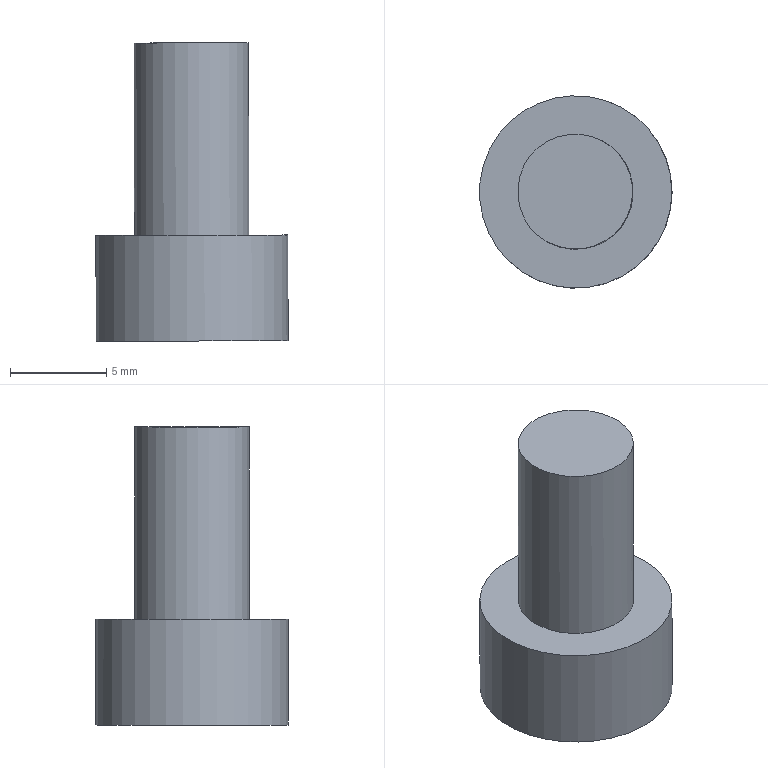Part | NX | features solid 2 | 1 solid | 12 faces | box 10.013 x 10.001 x 15.519 mm | volume 621.654 mm3 | plane 10 | spline 1 | cylinder 1 | commonest cylinder face diameters 10 x1
STEP:
#1=CARTESIAN_POINT('',(-491.131,18.224,140.018));
#2=VERTEX_POINT('',#1);
#3=CARTESIAN_POINT('',(-492.412,20.286,140.015));
#4=CARTESIAN_POINT('',(-491.355,17.975,140.017));
#5=CARTESIAN_POINT('',(-488.952,17.156,140.023));
#6=CARTESIAN_POINT('',(-486.649,18.209,140.028));
#7=CARTESIAN_POINT('',(-485.825,20.612,140.031));
#8=CARTESIAN_POINT('',(-486.88,22.919,140.029));
#9=CARTESIAN_POINT('',(-489.28,23.741,140.023));
#10=CARTESIAN_POINT('',(-491.587,22.69,140.018));
#11=CARTESIAN_POINT('',(-492.412,20.286,140.015));
#12=CARTESIAN_POINT('',(-491.355,17.975,140.017));
#13=CARTESIAN_POINT('',(-488.952,17.156,140.023));
#14=B_SPLINE_CURVE_WITH_KNOTS('',3,(#3,#4,#5,#6,#7,#8,#9,#10,#11,#12,#13),.UNSPECIFIED.,.T.,.F.,(1,1,1,1,1,1,1,1,1,1,1,1,1,1,1),(-0.007013,-0.004676,-0.002338,0.,0.002338,0.004676,0.007013,0.009351,0.01169,0.01403,0.01636,0.0187,0.02104,0.02338,0.02572),.UNSPECIFIED.);
#15=EDGE_CURVE('',#2,#2,#14,.T.);
#16=ORIENTED_EDGE('',*,*,#15,.F.);
#17=EDGE_LOOP('',(#16));
#18=FACE_BOUND('',#17,.T.);
#19=CARTESIAN_POINT('',(-491.107,18.226,130.018));
#20=VERTEX_POINT('',#19);
#21=CARTESIAN_POINT('',(-492.388,20.288,130.015));
#22=CARTESIAN_POINT('',(-491.332,17.977,130.017));
#23=CARTESIAN_POINT('',(-488.928,17.158,130.023));
#24=CARTESIAN_POINT('',(-486.625,18.211,130.029));
#25=CARTESIAN_POINT('',(-485.801,20.614,130.031));
#26=CARTESIAN_POINT('',(-486.856,22.921,130.029));
#27=CARTESIAN_POINT('',(-489.256,23.743,130.023));
#28=CARTESIAN_POINT('',(-491.563,22.692,130.018));
#29=CARTESIAN_POINT('',(-492.388,20.288,130.015));
#30=CARTESIAN_POINT('',(-491.332,17.977,130.017));
#31=CARTESIAN_POINT('',(-488.928,17.158,130.023));
#32=B_SPLINE_CURVE_WITH_KNOTS('',3,(#21,#22,#23,#24,#25,#26,#27,#28,#29,#30,#31),.UNSPECIFIED.,.T.,.F.,(1,1,1,1,1,1,1,1,1,1,1,1,1,1,1),(-0.007013,-0.004676,-0.002338,0.,0.002338,0.004676,0.007013,0.009351,0.01169,0.01403,0.01636,0.0187,0.02104,0.02338,0.02572),.UNSPECIFIED.);
#33=EDGE_CURVE('',#20,#20,#32,.T.);
#34=ORIENTED_EDGE('',*,*,#33,.T.);
#35=EDGE_LOOP('',(#34));
#36=FACE_BOUND('',#35,.T.);
#37=CARTESIAN_POINT('',(-485.825,20.613,140.031));
#38=CARTESIAN_POINT('',(-485.802,20.615,130.031));
#39=CARTESIAN_POINT('',(-486.881,22.921,140.029));
#40=CARTESIAN_POINT('',(-486.857,22.923,130.029));
#41=CARTESIAN_POINT('',(-489.283,23.741,140.023));
#42=CARTESIAN_POINT('',(-489.259,23.743,130.023));
#43=CARTESIAN_POINT('',(-491.591,22.685,140.018));
#44=CARTESIAN_POINT('',(-491.567,22.687,130.018));
#45=CARTESIAN_POINT('',(-492.411,20.284,140.015));
#46=CARTESIAN_POINT('',(-492.387,20.286,130.015));
#47=CARTESIAN_POINT('',(-491.355,17.976,140.017));
#48=CARTESIAN_POINT('',(-491.331,17.978,130.017));
#49=CARTESIAN_POINT('',(-488.954,17.155,140.023));
#50=CARTESIAN_POINT('',(-488.93,17.157,130.023));
#51=CARTESIAN_POINT('',(-486.646,18.211,140.029));
#52=CARTESIAN_POINT('',(-486.622,18.213,130.029));
#53=CARTESIAN_POINT('',(-485.825,20.613,140.031));
#54=CARTESIAN_POINT('',(-485.802,20.615,130.031));
#55=CARTESIAN_POINT('',(-486.881,22.921,140.029));
#56=CARTESIAN_POINT('',(-486.857,22.923,130.029));
#57=CARTESIAN_POINT('',(-489.283,23.741,140.023));
#58=CARTESIAN_POINT('',(-489.259,23.743,130.023));
#59=B_SPLINE_SURFACE_WITH_KNOTS('',3,1,((#37,#38),(#39,#40),(#41,#42),(#43,#44),(#45,#46),(#47,#48),(#49,#50),(#51,#52),(#53,#54),(#55,#56),(#57,#58)),.SURF_OF_LINEAR_EXTRUSION.,.T.,.F.,.F.,(1,1,1,1,1,1,1,1,1,1,1,1,1,1,1),(2,2),(-0.375,-0.25,-0.125,0.,0.125,0.25,0.375,0.5,0.625,0.75,0.875,1.,1.125,1.25,1.375),(0.,1.),.UNSPECIFIED.);
#60=ADVANCED_FACE('',(#18,#36),#59,.F.);
#61=ORIENTED_EDGE('',*,*,#15,.T.);
#62=EDGE_LOOP('',(#61));
#63=FACE_BOUND('',#62,.T.);
#64=CARTESIAN_POINT('',(-491.802,17.482,140.016));
#65=DIRECTION('',(-0.002392,-0.0002093,1.));
#66=DIRECTION('',(-0.7415,0.6709,-0.001634));
#67=AXIS2_PLACEMENT_3D('',#64,#65,#66);
#68=PLANE('',#67);
#69=ADVANCED_FACE('',(#63),#68,.T.);
#70=CARTESIAN_POINT('',(-494.075,20.015,130.011));
#71=VERTEX_POINT('',#70);
#72=CARTESIAN_POINT('',(-489.094,20.45,130.023));
#73=DIRECTION('',(-0.002392,-0.0002093,1.));
#74=DIRECTION('',(-0.9962,-0.08716,-0.002401));
#75=AXIS2_PLACEMENT_3D('',#72,#73,#74);
#76=CIRCLE('',#75,5.);
#77=EDGE_CURVE('',#71,#71,#76,.T.);
#78=ORIENTED_EDGE('',*,*,#77,.F.);
#79=EDGE_LOOP('',(#78));
#80=FACE_BOUND('',#79,.T.);
#81=CARTESIAN_POINT('',(-494.062,20.016,124.511));
#82=VERTEX_POINT('',#81);
#83=CARTESIAN_POINT('',(-489.081,20.452,124.523));
#84=DIRECTION('',(-0.002392,-0.0002093,1.));
#85=DIRECTION('',(-0.9962,-0.08716,-0.002401));
#86=AXIS2_PLACEMENT_3D('',#83,#84,#85);
#87=CIRCLE('',#86,5.);
#88=EDGE_CURVE('',#82,#82,#87,.T.);
#89=ORIENTED_EDGE('',*,*,#88,.T.);
#90=EDGE_LOOP('',(#89));
#91=FACE_BOUND('',#90,.T.);
#92=CARTESIAN_POINT('',(-489.094,20.45,130.023));
#93=DIRECTION('',(0.002392,0.0002093,-1.));
#94=DIRECTION('',(0.7415,-0.6709,0.001634));
#95=AXIS2_PLACEMENT_3D('',#92,#93,#94);
#96=CYLINDRICAL_SURFACE('',#95,5.);
#97=ADVANCED_FACE('',(#80,#91),#96,.T.);
#98=ORIENTED_EDGE('',*,*,#33,.F.);
#99=EDGE_LOOP('',(#98));
#100=FACE_BOUND('',#99,.T.);
#101=ORIENTED_EDGE('',*,*,#77,.T.);
#102=EDGE_LOOP('',(#101));
#103=FACE_BOUND('',#102,.T.);
#104=CARTESIAN_POINT('',(-489.094,20.45,130.023));
#105=DIRECTION('',(0.002392,0.0002093,-1.));
#106=DIRECTION('',(0.7415,-0.6709,0.001634));
#107=AXIS2_PLACEMENT_3D('',#104,#105,#106);
#108=PLANE('',#107);
#109=ADVANCED_FACE('',(#100,#103),#108,.F.);
#110=CARTESIAN_POINT('',(-491.205,18.104,124.518));
#111=VERTEX_POINT('',#110);
#112=CARTESIAN_POINT('',(-488.11,17.439,124.525));
#113=VERTEX_POINT('',#112);
#114=CARTESIAN_POINT('',(-489.658,17.772,124.521));
#115=DIRECTION('',(0.9776,-0.2103,0.002295));
#116=VECTOR('',#115,1000.);
#117=LINE('',#114,#116);
#118=EDGE_CURVE('',#111,#113,#117,.T.);
#119=ORIENTED_EDGE('',*,*,#118,.T.);
#120=CARTESIAN_POINT('',(-485.987,19.786,124.53));
#121=VERTEX_POINT('',#120);
#122=CARTESIAN_POINT('',(-487.049,18.612,124.528));
#123=DIRECTION('',(0.6709,0.7415,0.00176));
#124=VECTOR('',#123,1000.);
#125=LINE('',#122,#124);
#126=EDGE_CURVE('',#113,#121,#125,.T.);
#127=ORIENTED_EDGE('',*,*,#126,.T.);
#128=CARTESIAN_POINT('',(-486.958,22.799,124.529));
#129=VERTEX_POINT('',#128);
#130=CARTESIAN_POINT('',(-486.472,21.292,124.53));
#131=DIRECTION('',(-0.3067,0.9518,-0.0005346));
#132=VECTOR('',#131,1000.);
#133=LINE('',#130,#132);
#134=EDGE_CURVE('',#121,#129,#133,.T.);
#135=ORIENTED_EDGE('',*,*,#134,.T.);
#136=CARTESIAN_POINT('',(-490.052,23.464,124.521));
#137=VERTEX_POINT('',#136);
#138=CARTESIAN_POINT('',(-488.505,23.132,124.525));
#139=DIRECTION('',(-0.9776,0.2103,-0.002295));
#140=VECTOR('',#139,1000.);
#141=LINE('',#138,#140);
#142=EDGE_CURVE('',#129,#137,#141,.T.);
#143=ORIENTED_EDGE('',*,*,#142,.T.);
#144=CARTESIAN_POINT('',(-492.176,21.117,124.516));
#145=VERTEX_POINT('',#144);
#146=CARTESIAN_POINT('',(-491.114,22.291,124.519));
#147=DIRECTION('',(-0.6709,-0.7415,-0.00176));
#148=VECTOR('',#147,1000.);
#149=LINE('',#146,#148);
#150=EDGE_CURVE('',#137,#145,#149,.T.);
#151=ORIENTED_EDGE('',*,*,#150,.T.);
#152=CARTESIAN_POINT('',(-491.69,19.611,124.517));
#153=DIRECTION('',(0.3067,-0.9518,0.0005346));
#154=VECTOR('',#153,1000.);
#155=LINE('',#152,#154);
#156=EDGE_CURVE('',#145,#111,#155,.T.);
#157=ORIENTED_EDGE('',*,*,#156,.T.);
#158=EDGE_LOOP('',(#119,#127,#135,#143,#151,#157));
#159=FACE_BOUND('',#158,.T.);
#160=ORIENTED_EDGE('',*,*,#88,.F.);
#161=EDGE_LOOP('',(#160));
#162=FACE_BOUND('',#161,.T.);
#163=CARTESIAN_POINT('',(-489.081,20.452,124.523));
#164=DIRECTION('',(0.002392,0.0002093,-1.));
#165=DIRECTION('',(0.7415,-0.6709,0.001634));
#166=AXIS2_PLACEMENT_3D('',#163,#164,#165);
#167=PLANE('',#166);
#168=ADVANCED_FACE('',(#159,#162),#167,.T.);
#169=ORIENTED_EDGE('',*,*,#118,.F.);
#170=CARTESIAN_POINT('',(-491.213,18.104,128.018));
#171=VERTEX_POINT('',#170);
#172=CARTESIAN_POINT('',(-491.213,18.104,128.018));
#173=DIRECTION('',(0.002392,0.0002093,-1.));
#174=VECTOR('',#173,1000.);
#175=LINE('',#172,#174);
#176=EDGE_CURVE('',#171,#111,#175,.T.);
#177=ORIENTED_EDGE('',*,*,#176,.F.);
#178=CARTESIAN_POINT('',(-488.119,17.438,128.025));
#179=VERTEX_POINT('',#178);
#180=CARTESIAN_POINT('',(-491.778,18.225,128.016));
#181=DIRECTION('',(0.9776,-0.2103,0.002295));
#182=VECTOR('',#181,1000.);
#183=LINE('',#180,#182);
#184=EDGE_CURVE('',#171,#179,#183,.T.);
#185=ORIENTED_EDGE('',*,*,#184,.T.);
#186=CARTESIAN_POINT('',(-488.119,17.438,128.025));
#187=DIRECTION('',(0.002392,0.0002093,-1.));
#188=VECTOR('',#187,1000.);
#189=LINE('',#186,#188);
#190=EDGE_CURVE('',#179,#113,#189,.T.);
#191=ORIENTED_EDGE('',*,*,#190,.T.);
#192=EDGE_LOOP('',(#169,#177,#185,#191));
#193=FACE_BOUND('',#192,.T.);
#194=CARTESIAN_POINT('',(-491.778,18.225,128.016));
#195=DIRECTION('',(-0.2103,-0.9776,-0.0007076));
#196=DIRECTION('',(-0.9776,0.2103,-0.002295));
#197=AXIS2_PLACEMENT_3D('',#194,#195,#196);
#198=PLANE('',#197);
#199=ADVANCED_FACE('',(#193),#198,.F.);
#200=ORIENTED_EDGE('',*,*,#126,.F.);
#201=ORIENTED_EDGE('',*,*,#190,.F.);
#202=CARTESIAN_POINT('',(-485.995,19.785,128.03));
#203=VERTEX_POINT('',#202);
#204=CARTESIAN_POINT('',(-488.506,17.01,128.024));
#205=DIRECTION('',(0.6709,0.7415,0.00176));
#206=VECTOR('',#205,1000.);
#207=LINE('',#204,#206);
#208=EDGE_CURVE('',#179,#203,#207,.T.);
#209=ORIENTED_EDGE('',*,*,#208,.T.);
#210=CARTESIAN_POINT('',(-485.995,19.785,128.03));
#211=DIRECTION('',(0.002392,0.0002093,-1.));
#212=VECTOR('',#211,1000.);
#213=LINE('',#210,#212);
#214=EDGE_CURVE('',#203,#121,#213,.T.);
#215=ORIENTED_EDGE('',*,*,#214,.T.);
#216=EDGE_LOOP('',(#200,#201,#209,#215));
#217=FACE_BOUND('',#216,.T.);
#218=CARTESIAN_POINT('',(-488.506,17.01,128.024));
#219=DIRECTION('',(0.7415,-0.6709,0.001634));
#220=DIRECTION('',(-0.6709,-0.7415,-0.00176));
#221=AXIS2_PLACEMENT_3D('',#218,#219,#220);
#222=PLANE('',#221);
#223=ADVANCED_FACE('',(#217),#222,.F.);
#224=ORIENTED_EDGE('',*,*,#134,.F.);
#225=ORIENTED_EDGE('',*,*,#214,.F.);
#226=CARTESIAN_POINT('',(-486.966,22.798,128.029));
#227=VERTEX_POINT('',#226);
#228=CARTESIAN_POINT('',(-485.818,19.236,128.031));
#229=DIRECTION('',(-0.3067,0.9518,-0.0005346));
#230=VECTOR('',#229,1000.);
#231=LINE('',#228,#230);
#232=EDGE_CURVE('',#203,#227,#231,.T.);
#233=ORIENTED_EDGE('',*,*,#232,.T.);
#234=CARTESIAN_POINT('',(-486.966,22.798,128.029));
#235=DIRECTION('',(0.002392,0.0002093,-1.));
#236=VECTOR('',#235,1000.);
#237=LINE('',#234,#236);
#238=EDGE_CURVE('',#227,#129,#237,.T.);
#239=ORIENTED_EDGE('',*,*,#238,.T.);
#240=EDGE_LOOP('',(#224,#225,#233,#239));
#241=FACE_BOUND('',#240,.T.);
#242=CARTESIAN_POINT('',(-485.818,19.236,128.031));
#243=DIRECTION('',(0.9518,0.3067,0.002341));
#244=DIRECTION('',(0.3067,-0.9518,0.0005346));
#245=AXIS2_PLACEMENT_3D('',#242,#243,#244);
#246=PLANE('',#245);
#247=ADVANCED_FACE('',(#241),#246,.F.);
#248=ORIENTED_EDGE('',*,*,#142,.F.);
#249=ORIENTED_EDGE('',*,*,#238,.F.);
#250=CARTESIAN_POINT('',(-490.061,23.464,128.021));
#251=VERTEX_POINT('',#250);
#252=CARTESIAN_POINT('',(-486.402,22.677,128.03));
#253=DIRECTION('',(-0.9776,0.2103,-0.002295));
#254=VECTOR('',#253,1000.);
#255=LINE('',#252,#254);
#256=EDGE_CURVE('',#227,#251,#255,.T.);
#257=ORIENTED_EDGE('',*,*,#256,.T.);
#258=CARTESIAN_POINT('',(-490.061,23.464,128.021));
#259=DIRECTION('',(0.002392,0.0002093,-1.));
#260=VECTOR('',#259,1000.);
#261=LINE('',#258,#260);
#262=EDGE_CURVE('',#251,#137,#261,.T.);
#263=ORIENTED_EDGE('',*,*,#262,.T.);
#264=EDGE_LOOP('',(#248,#249,#257,#263));
#265=FACE_BOUND('',#264,.T.);
#266=CARTESIAN_POINT('',(-486.402,22.677,128.03));
#267=DIRECTION('',(0.2103,0.9776,0.0007076));
#268=DIRECTION('',(0.9776,-0.2103,0.002295));
#269=AXIS2_PLACEMENT_3D('',#266,#267,#268);
#270=PLANE('',#269);
#271=ADVANCED_FACE('',(#265),#270,.F.);
#272=ORIENTED_EDGE('',*,*,#150,.F.);
#273=ORIENTED_EDGE('',*,*,#262,.F.);
#274=CARTESIAN_POINT('',(-492.184,21.116,128.016));
#275=VERTEX_POINT('',#274);
#276=CARTESIAN_POINT('',(-489.673,23.892,128.022));
#277=DIRECTION('',(-0.6709,-0.7415,-0.00176));
#278=VECTOR('',#277,1000.);
#279=LINE('',#276,#278);
#280=EDGE_CURVE('',#251,#275,#279,.T.);
#281=ORIENTED_EDGE('',*,*,#280,.T.);
#282=CARTESIAN_POINT('',(-492.184,21.116,128.016));
#283=DIRECTION('',(0.002392,0.0002093,-1.));
#284=VECTOR('',#283,1000.);
#285=LINE('',#282,#284);
#286=EDGE_CURVE('',#275,#145,#285,.T.);
#287=ORIENTED_EDGE('',*,*,#286,.T.);
#288=EDGE_LOOP('',(#272,#273,#281,#287));
#289=FACE_BOUND('',#288,.T.);
#290=CARTESIAN_POINT('',(-489.673,23.892,128.022));
#291=DIRECTION('',(-0.7415,0.6709,-0.001634));
#292=DIRECTION('',(0.6709,0.7415,0.00176));
#293=AXIS2_PLACEMENT_3D('',#290,#291,#292);
#294=PLANE('',#293);
#295=ADVANCED_FACE('',(#289),#294,.F.);
#296=ORIENTED_EDGE('',*,*,#156,.F.);
#297=ORIENTED_EDGE('',*,*,#286,.F.);
#298=CARTESIAN_POINT('',(-492.361,21.666,128.016));
#299=DIRECTION('',(0.3067,-0.9518,0.0005346));
#300=VECTOR('',#299,1000.);
#301=LINE('',#298,#300);
#302=EDGE_CURVE('',#275,#171,#301,.T.);
#303=ORIENTED_EDGE('',*,*,#302,.T.);
#304=ORIENTED_EDGE('',*,*,#176,.T.);
#305=EDGE_LOOP('',(#296,#297,#303,#304));
#306=FACE_BOUND('',#305,.T.);
#307=CARTESIAN_POINT('',(-492.361,21.666,128.016));
#308=DIRECTION('',(-0.9518,-0.3067,-0.002341));
#309=DIRECTION('',(-0.3067,0.9518,-0.0005346));
#310=AXIS2_PLACEMENT_3D('',#307,#308,#309);
#311=PLANE('',#310);
#312=ADVANCED_FACE('',(#306),#311,.F.);
#313=ORIENTED_EDGE('',*,*,#184,.F.);
#314=ORIENTED_EDGE('',*,*,#302,.F.);
#315=ORIENTED_EDGE('',*,*,#280,.F.);
#316=ORIENTED_EDGE('',*,*,#256,.F.);
#317=ORIENTED_EDGE('',*,*,#232,.F.);
#318=ORIENTED_EDGE('',*,*,#208,.F.);
#319=EDGE_LOOP('',(#313,#314,#315,#316,#317,#318));
#320=FACE_BOUND('',#319,.T.);
#321=CARTESIAN_POINT('',(-496.211,18.156,128.006));
#322=DIRECTION('',(-0.002392,-0.0002093,1.));
#323=DIRECTION('',(-0.7415,0.6709,-0.001634));
#324=AXIS2_PLACEMENT_3D('',#321,#322,#323);
#325=PLANE('',#324);
#326=ADVANCED_FACE('',(#320),#325,.F.);
#327=CLOSED_SHELL('',(#60,#69,#97,#109,#168,#199,#223,#247,#271,#295,#312,#326));
#328=MANIFOLD_SOLID_BREP('',#327);
#329=(LENGTH_UNIT()NAMED_UNIT(*)SI_UNIT(.MILLI.,.METRE.));
#330=UNCERTAINTY_MEASURE_WITH_UNIT(LENGTH_MEASURE(0.0508),#329,'','');
#331=(NAMED_UNIT(*)PLANE_ANGLE_UNIT()SI_UNIT($,.RADIAN.));
#332=(NAMED_UNIT(*)SI_UNIT($,.STERADIAN.)SOLID_ANGLE_UNIT());
#333=(GEOMETRIC_REPRESENTATION_CONTEXT(3)GLOBAL_UNCERTAINTY_ASSIGNED_CONTEXT((#330))GLOBAL_UNIT_ASSIGNED_CONTEXT((#329,#331,#332))REPRESENTATION_CONTEXT('',''));
#334=ADVANCED_BREP_SHAPE_REPRESENTATION('',(#328),#333);